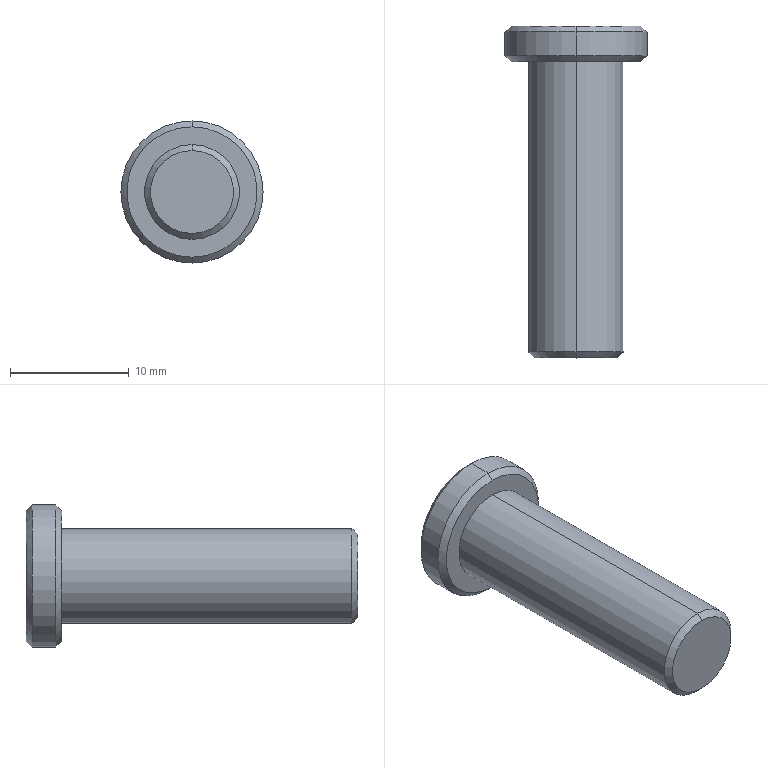Part | SolidWorks | features Chamfer 1, Extrusion 1, ICE 1 | 1 solid | 13 faces | box 12 x 28 x 12 mm | volume 1584 mm3 | cone 6 | cylinder 4 | plane 3 | commonest cylinder face diameters 8 x2 12 x2
STEP:
#1=CARTESIAN_POINT('',(0.,28.,5.5));
#2=VERTEX_POINT('',#1);
#3=CARTESIAN_POINT('',(0.,28.,-5.5));
#4=VERTEX_POINT('',#3);
#5=CARTESIAN_POINT('',(0.,28.,0.));
#6=DIRECTION('',(0.,1.,0.));
#7=DIRECTION('',(0.,0.,1.));
#8=AXIS2_PLACEMENT_3D('',#5,#6,#7);
#9=CIRCLE('',#8,5.5);
#10=EDGE_CURVE('',#2,#4,#9,.T.);
#11=ORIENTED_EDGE('',*,*,#10,.F.);
#12=CARTESIAN_POINT('',(0.,27.5,6.));
#13=VERTEX_POINT('',#12);
#14=CARTESIAN_POINT('',(0.,28.,5.5));
#15=DIRECTION('',(0.,-0.7071,0.7071));
#16=VECTOR('',#15,1000.);
#17=LINE('',#14,#16);
#18=EDGE_CURVE('',#2,#13,#17,.T.);
#19=ORIENTED_EDGE('',*,*,#18,.T.);
#20=CARTESIAN_POINT('',(0.,27.5,-6.));
#21=VERTEX_POINT('',#20);
#22=CARTESIAN_POINT('',(0.,27.5,0.));
#23=DIRECTION('',(0.,-1.,0.));
#24=DIRECTION('',(0.,0.,1.));
#25=AXIS2_PLACEMENT_3D('',#22,#23,#24);
#26=CIRCLE('',#25,6.);
#27=EDGE_CURVE('',#21,#13,#26,.T.);
#28=ORIENTED_EDGE('',*,*,#27,.F.);
#29=CARTESIAN_POINT('',(0.,28.,-5.5));
#30=DIRECTION('',(0.,-0.7071,-0.7071));
#31=VECTOR('',#30,1000.);
#32=LINE('',#29,#31);
#33=EDGE_CURVE('',#4,#21,#32,.T.);
#34=ORIENTED_EDGE('',*,*,#33,.F.);
#35=EDGE_LOOP('',(#11,#19,#28,#34));
#36=FACE_OUTER_BOUND('',#35,.T.);
#37=CARTESIAN_POINT('',(0.,28.,0.));
#38=DIRECTION('',(0.,-1.,0.));
#39=DIRECTION('',(0.,0.,-1.));
#40=AXIS2_PLACEMENT_3D('',#37,#38,#39);
#41=CONICAL_SURFACE('',#40,5.5,0.7854);
#42=ADVANCED_FACE('',(#36),#41,.T.);
#43=CARTESIAN_POINT('',(0.,25.,-5.5));
#44=VERTEX_POINT('',#43);
#45=CARTESIAN_POINT('',(0.,25.,5.5));
#46=VERTEX_POINT('',#45);
#47=CARTESIAN_POINT('',(0.,25.,0.));
#48=DIRECTION('',(0.,-1.,0.));
#49=DIRECTION('',(0.,0.,1.));
#50=AXIS2_PLACEMENT_3D('',#47,#48,#49);
#51=CIRCLE('',#50,5.5);
#52=EDGE_CURVE('',#44,#46,#51,.T.);
#53=ORIENTED_EDGE('',*,*,#52,.F.);
#54=CARTESIAN_POINT('',(0.,25.5,-6.));
#55=VERTEX_POINT('',#54);
#56=CARTESIAN_POINT('',(0.,25.5,-6.));
#57=DIRECTION('',(0.,0.7071,-0.7071));
#58=VECTOR('',#57,1000.);
#59=LINE('',#56,#58);
#60=EDGE_CURVE('',#44,#55,#59,.T.);
#61=ORIENTED_EDGE('',*,*,#60,.T.);
#62=CARTESIAN_POINT('',(0.,25.5,6.));
#63=VERTEX_POINT('',#62);
#64=CARTESIAN_POINT('',(0.,25.5,0.));
#65=DIRECTION('',(0.,1.,0.));
#66=DIRECTION('',(0.,0.,1.));
#67=AXIS2_PLACEMENT_3D('',#64,#65,#66);
#68=CIRCLE('',#67,6.);
#69=EDGE_CURVE('',#63,#55,#68,.T.);
#70=ORIENTED_EDGE('',*,*,#69,.F.);
#71=CARTESIAN_POINT('',(0.,25.5,6.));
#72=DIRECTION('',(0.,0.7071,0.7071));
#73=VECTOR('',#72,1000.);
#74=LINE('',#71,#73);
#75=EDGE_CURVE('',#46,#63,#74,.T.);
#76=ORIENTED_EDGE('',*,*,#75,.F.);
#77=EDGE_LOOP('',(#53,#61,#70,#76));
#78=FACE_OUTER_BOUND('',#77,.T.);
#79=CARTESIAN_POINT('',(0.,25.5,0.));
#80=DIRECTION('',(0.,1.,0.));
#81=DIRECTION('',(0.,0.,1.));
#82=AXIS2_PLACEMENT_3D('',#79,#80,#81);
#83=CONICAL_SURFACE('',#82,6.,0.7854);
#84=ADVANCED_FACE('',(#78),#83,.T.);
#85=CARTESIAN_POINT('',(0.,0.,-3.5));
#86=VERTEX_POINT('',#85);
#87=CARTESIAN_POINT('',(0.,0.,3.5));
#88=VERTEX_POINT('',#87);
#89=CARTESIAN_POINT('',(0.,0.,0.));
#90=DIRECTION('',(0.,-1.,0.));
#91=DIRECTION('',(0.,0.,1.));
#92=AXIS2_PLACEMENT_3D('',#89,#90,#91);
#93=CIRCLE('',#92,3.5);
#94=EDGE_CURVE('',#86,#88,#93,.T.);
#95=ORIENTED_EDGE('',*,*,#94,.F.);
#96=CARTESIAN_POINT('',(0.,0.5,-4.));
#97=VERTEX_POINT('',#96);
#98=CARTESIAN_POINT('',(0.,0.5,-4.));
#99=DIRECTION('',(0.,0.7071,-0.7071));
#100=VECTOR('',#99,1000.);
#101=LINE('',#98,#100);
#102=EDGE_CURVE('',#86,#97,#101,.T.);
#103=ORIENTED_EDGE('',*,*,#102,.T.);
#104=CARTESIAN_POINT('',(0.,0.5,4.));
#105=VERTEX_POINT('',#104);
#106=CARTESIAN_POINT('',(0.,0.5,0.));
#107=DIRECTION('',(0.,1.,0.));
#108=DIRECTION('',(0.,0.,1.));
#109=AXIS2_PLACEMENT_3D('',#106,#107,#108);
#110=CIRCLE('',#109,4.);
#111=EDGE_CURVE('',#105,#97,#110,.T.);
#112=ORIENTED_EDGE('',*,*,#111,.F.);
#113=CARTESIAN_POINT('',(0.,0.5,4.));
#114=DIRECTION('',(0.,0.7071,0.7071));
#115=VECTOR('',#114,1000.);
#116=LINE('',#113,#115);
#117=EDGE_CURVE('',#88,#105,#116,.T.);
#118=ORIENTED_EDGE('',*,*,#117,.F.);
#119=EDGE_LOOP('',(#95,#103,#112,#118));
#120=FACE_OUTER_BOUND('',#119,.T.);
#121=CARTESIAN_POINT('',(0.,0.5,0.));
#122=DIRECTION('',(0.,1.,0.));
#123=DIRECTION('',(0.,0.,1.));
#124=AXIS2_PLACEMENT_3D('',#121,#122,#123);
#125=CONICAL_SURFACE('',#124,4.,0.7854);
#126=ADVANCED_FACE('',(#120),#125,.T.);
#127=ORIENTED_EDGE('',*,*,#27,.T.);
#128=CARTESIAN_POINT('',(0.,28.,6.));
#129=DIRECTION('',(0.,-1.,0.));
#130=VECTOR('',#129,1000.);
#131=LINE('',#128,#130);
#132=EDGE_CURVE('',#13,#63,#131,.T.);
#133=ORIENTED_EDGE('',*,*,#132,.T.);
#134=ORIENTED_EDGE('',*,*,#69,.T.);
#135=CARTESIAN_POINT('',(0.,28.,-6.));
#136=DIRECTION('',(0.,-1.,0.));
#137=VECTOR('',#136,1000.);
#138=LINE('',#135,#137);
#139=EDGE_CURVE('',#21,#55,#138,.T.);
#140=ORIENTED_EDGE('',*,*,#139,.F.);
#141=EDGE_LOOP('',(#127,#133,#134,#140));
#142=FACE_OUTER_BOUND('',#141,.T.);
#143=CARTESIAN_POINT('',(0.,28.,0.));
#144=DIRECTION('',(0.,-1.,0.));
#145=DIRECTION('',(0.,0.,-1.));
#146=AXIS2_PLACEMENT_3D('',#143,#144,#145);
#147=CYLINDRICAL_SURFACE('',#146,6.);
#148=ADVANCED_FACE('',(#142),#147,.T.);
#149=CARTESIAN_POINT('',(0.,25.,4.));
#150=VERTEX_POINT('',#149);
#151=CARTESIAN_POINT('',(0.,25.,-4.));
#152=VERTEX_POINT('',#151);
#153=CARTESIAN_POINT('',(0.,25.,0.));
#154=DIRECTION('',(0.,1.,0.));
#155=DIRECTION('',(0.,0.,1.));
#156=AXIS2_PLACEMENT_3D('',#153,#154,#155);
#157=CIRCLE('',#156,4.);
#158=EDGE_CURVE('',#150,#152,#157,.T.);
#159=ORIENTED_EDGE('',*,*,#158,.F.);
#160=CARTESIAN_POINT('',(0.,25.,4.));
#161=DIRECTION('',(0.,-1.,0.));
#162=VECTOR('',#161,1000.);
#163=LINE('',#160,#162);
#164=EDGE_CURVE('',#150,#105,#163,.T.);
#165=ORIENTED_EDGE('',*,*,#164,.T.);
#166=ORIENTED_EDGE('',*,*,#111,.T.);
#167=CARTESIAN_POINT('',(0.,25.,-4.));
#168=DIRECTION('',(0.,-1.,0.));
#169=VECTOR('',#168,1000.);
#170=LINE('',#167,#169);
#171=EDGE_CURVE('',#152,#97,#170,.T.);
#172=ORIENTED_EDGE('',*,*,#171,.F.);
#173=EDGE_LOOP('',(#159,#165,#166,#172));
#174=FACE_OUTER_BOUND('',#173,.T.);
#175=CARTESIAN_POINT('',(0.,25.,0.));
#176=DIRECTION('',(0.,-1.,0.));
#177=DIRECTION('',(0.,0.,-1.));
#178=AXIS2_PLACEMENT_3D('',#175,#176,#177);
#179=CYLINDRICAL_SURFACE('',#178,4.);
#180=ADVANCED_FACE('',(#174),#179,.T.);
#181=ORIENTED_EDGE('',*,*,#164,.F.);
#182=CARTESIAN_POINT('',(0.,25.,0.));
#183=DIRECTION('',(0.,1.,0.));
#184=DIRECTION('',(0.,0.,1.));
#185=AXIS2_PLACEMENT_3D('',#182,#183,#184);
#186=CIRCLE('',#185,4.);
#187=EDGE_CURVE('',#152,#150,#186,.T.);
#188=ORIENTED_EDGE('',*,*,#187,.F.);
#189=ORIENTED_EDGE('',*,*,#171,.T.);
#190=CARTESIAN_POINT('',(0.,0.5,0.));
#191=DIRECTION('',(0.,1.,0.));
#192=DIRECTION('',(0.,0.,1.));
#193=AXIS2_PLACEMENT_3D('',#190,#191,#192);
#194=CIRCLE('',#193,4.);
#195=EDGE_CURVE('',#97,#105,#194,.T.);
#196=ORIENTED_EDGE('',*,*,#195,.T.);
#197=EDGE_LOOP('',(#181,#188,#189,#196));
#198=FACE_OUTER_BOUND('',#197,.T.);
#199=CARTESIAN_POINT('',(0.,25.,0.));
#200=DIRECTION('',(0.,-1.,0.));
#201=DIRECTION('',(0.,0.,-1.));
#202=AXIS2_PLACEMENT_3D('',#199,#200,#201);
#203=CYLINDRICAL_SURFACE('',#202,4.);
#204=ADVANCED_FACE('',(#198),#203,.T.);
#205=CARTESIAN_POINT('',(0.,0.,0.));
#206=DIRECTION('',(0.,-1.,0.));
#207=DIRECTION('',(0.,0.,1.));
#208=AXIS2_PLACEMENT_3D('',#205,#206,#207);
#209=CIRCLE('',#208,3.5);
#210=EDGE_CURVE('',#88,#86,#209,.T.);
#211=ORIENTED_EDGE('',*,*,#210,.T.);
#212=ORIENTED_EDGE('',*,*,#94,.T.);
#213=EDGE_LOOP('',(#211,#212));
#214=FACE_OUTER_BOUND('',#213,.T.);
#215=CARTESIAN_POINT('',(0.,0.,0.));
#216=DIRECTION('',(0.,1.,0.));
#217=DIRECTION('',(0.,0.,1.));
#218=AXIS2_PLACEMENT_3D('',#215,#216,#217);
#219=PLANE('',#218);
#220=ADVANCED_FACE('',(#214),#219,.F.);
#221=ORIENTED_EDGE('',*,*,#132,.F.);
#222=CARTESIAN_POINT('',(0.,27.5,0.));
#223=DIRECTION('',(0.,-1.,0.));
#224=DIRECTION('',(0.,0.,1.));
#225=AXIS2_PLACEMENT_3D('',#222,#223,#224);
#226=CIRCLE('',#225,6.);
#227=EDGE_CURVE('',#13,#21,#226,.T.);
#228=ORIENTED_EDGE('',*,*,#227,.T.);
#229=ORIENTED_EDGE('',*,*,#139,.T.);
#230=CARTESIAN_POINT('',(0.,25.5,0.));
#231=DIRECTION('',(0.,1.,0.));
#232=DIRECTION('',(0.,0.,1.));
#233=AXIS2_PLACEMENT_3D('',#230,#231,#232);
#234=CIRCLE('',#233,6.);
#235=EDGE_CURVE('',#55,#63,#234,.T.);
#236=ORIENTED_EDGE('',*,*,#235,.T.);
#237=EDGE_LOOP('',(#221,#228,#229,#236));
#238=FACE_OUTER_BOUND('',#237,.T.);
#239=CARTESIAN_POINT('',(0.,28.,0.));
#240=DIRECTION('',(0.,-1.,0.));
#241=DIRECTION('',(0.,0.,-1.));
#242=AXIS2_PLACEMENT_3D('',#239,#240,#241);
#243=CYLINDRICAL_SURFACE('',#242,6.);
#244=ADVANCED_FACE('',(#238),#243,.T.);
#245=CARTESIAN_POINT('',(0.,28.,0.));
#246=DIRECTION('',(0.,1.,0.));
#247=DIRECTION('',(0.,0.,1.));
#248=AXIS2_PLACEMENT_3D('',#245,#246,#247);
#249=CIRCLE('',#248,5.5);
#250=EDGE_CURVE('',#4,#2,#249,.T.);
#251=ORIENTED_EDGE('',*,*,#250,.T.);
#252=ORIENTED_EDGE('',*,*,#10,.T.);
#253=EDGE_LOOP('',(#251,#252));
#254=FACE_OUTER_BOUND('',#253,.T.);
#255=CARTESIAN_POINT('',(0.,28.,0.));
#256=DIRECTION('',(0.,1.,0.));
#257=DIRECTION('',(0.,0.,1.));
#258=AXIS2_PLACEMENT_3D('',#255,#256,#257);
#259=PLANE('',#258);
#260=ADVANCED_FACE('',(#254),#259,.T.);
#261=CARTESIAN_POINT('',(0.,25.,0.));
#262=DIRECTION('',(0.,-1.,0.));
#263=DIRECTION('',(0.,0.,1.));
#264=AXIS2_PLACEMENT_3D('',#261,#262,#263);
#265=CIRCLE('',#264,5.5);
#266=EDGE_CURVE('',#46,#44,#265,.T.);
#267=ORIENTED_EDGE('',*,*,#266,.T.);
#268=ORIENTED_EDGE('',*,*,#52,.T.);
#269=EDGE_LOOP('',(#267,#268));
#270=FACE_OUTER_BOUND('',#269,.T.);
#271=ORIENTED_EDGE('',*,*,#187,.T.);
#272=ORIENTED_EDGE('',*,*,#158,.T.);
#273=EDGE_LOOP('',(#271,#272));
#274=FACE_BOUND('',#273,.T.);
#275=CARTESIAN_POINT('',(0.,25.,0.));
#276=DIRECTION('',(0.,1.,0.));
#277=DIRECTION('',(0.,0.,1.));
#278=AXIS2_PLACEMENT_3D('',#275,#276,#277);
#279=PLANE('',#278);
#280=ADVANCED_FACE('',(#270,#274),#279,.F.);
#281=ORIENTED_EDGE('',*,*,#102,.F.);
#282=ORIENTED_EDGE('',*,*,#210,.F.);
#283=ORIENTED_EDGE('',*,*,#117,.T.);
#284=ORIENTED_EDGE('',*,*,#195,.F.);
#285=EDGE_LOOP('',(#281,#282,#283,#284));
#286=FACE_OUTER_BOUND('',#285,.T.);
#287=CARTESIAN_POINT('',(0.,0.5,0.));
#288=DIRECTION('',(0.,1.,0.));
#289=DIRECTION('',(0.,0.,1.));
#290=AXIS2_PLACEMENT_3D('',#287,#288,#289);
#291=CONICAL_SURFACE('',#290,4.,0.7854);
#292=ADVANCED_FACE('',(#286),#291,.T.);
#293=ORIENTED_EDGE('',*,*,#60,.F.);
#294=ORIENTED_EDGE('',*,*,#266,.F.);
#295=ORIENTED_EDGE('',*,*,#75,.T.);
#296=ORIENTED_EDGE('',*,*,#235,.F.);
#297=EDGE_LOOP('',(#293,#294,#295,#296));
#298=FACE_OUTER_BOUND('',#297,.T.);
#299=CARTESIAN_POINT('',(0.,25.5,0.));
#300=DIRECTION('',(0.,1.,0.));
#301=DIRECTION('',(0.,0.,1.));
#302=AXIS2_PLACEMENT_3D('',#299,#300,#301);
#303=CONICAL_SURFACE('',#302,6.,0.7854);
#304=ADVANCED_FACE('',(#298),#303,.T.);
#305=ORIENTED_EDGE('',*,*,#18,.F.);
#306=ORIENTED_EDGE('',*,*,#250,.F.);
#307=ORIENTED_EDGE('',*,*,#33,.T.);
#308=ORIENTED_EDGE('',*,*,#227,.F.);
#309=EDGE_LOOP('',(#305,#306,#307,#308));
#310=FACE_OUTER_BOUND('',#309,.T.);
#311=CARTESIAN_POINT('',(0.,28.,0.));
#312=DIRECTION('',(0.,-1.,0.));
#313=DIRECTION('',(0.,0.,-1.));
#314=AXIS2_PLACEMENT_3D('',#311,#312,#313);
#315=CONICAL_SURFACE('',#314,5.5,0.7854);
#316=ADVANCED_FACE('',(#310),#315,.T.);
#317=CLOSED_SHELL('',(#42,#84,#126,#148,#180,#204,#220,#244,#260,#280,#292,#304,#316));
#318=MANIFOLD_SOLID_BREP('',#317);
#319=CARTESIAN_POINT('',(0.,0.,0.));
#320=DIRECTION('',(0.,0.,1.));
#321=DIRECTION('',(1.,0.,0.));
#322=AXIS2_PLACEMENT_3D('',#319,#320,#321);
#323=(LENGTH_UNIT()NAMED_UNIT(*)SI_UNIT(.MILLI.,.METRE.));
#324=UNCERTAINTY_MEASURE_WITH_UNIT(LENGTH_MEASURE(0.00001),#323,'','');
#325=(NAMED_UNIT(*)PLANE_ANGLE_UNIT()SI_UNIT($,.RADIAN.));
#326=(NAMED_UNIT(*)SI_UNIT($,.STERADIAN.)SOLID_ANGLE_UNIT());
#327=(GEOMETRIC_REPRESENTATION_CONTEXT(3)GLOBAL_UNCERTAINTY_ASSIGNED_CONTEXT((#324))GLOBAL_UNIT_ASSIGNED_CONTEXT((#323,#325,#326))REPRESENTATION_CONTEXT('',''));
#328=ADVANCED_BREP_SHAPE_REPRESENTATION('',(#318,#322),#327);